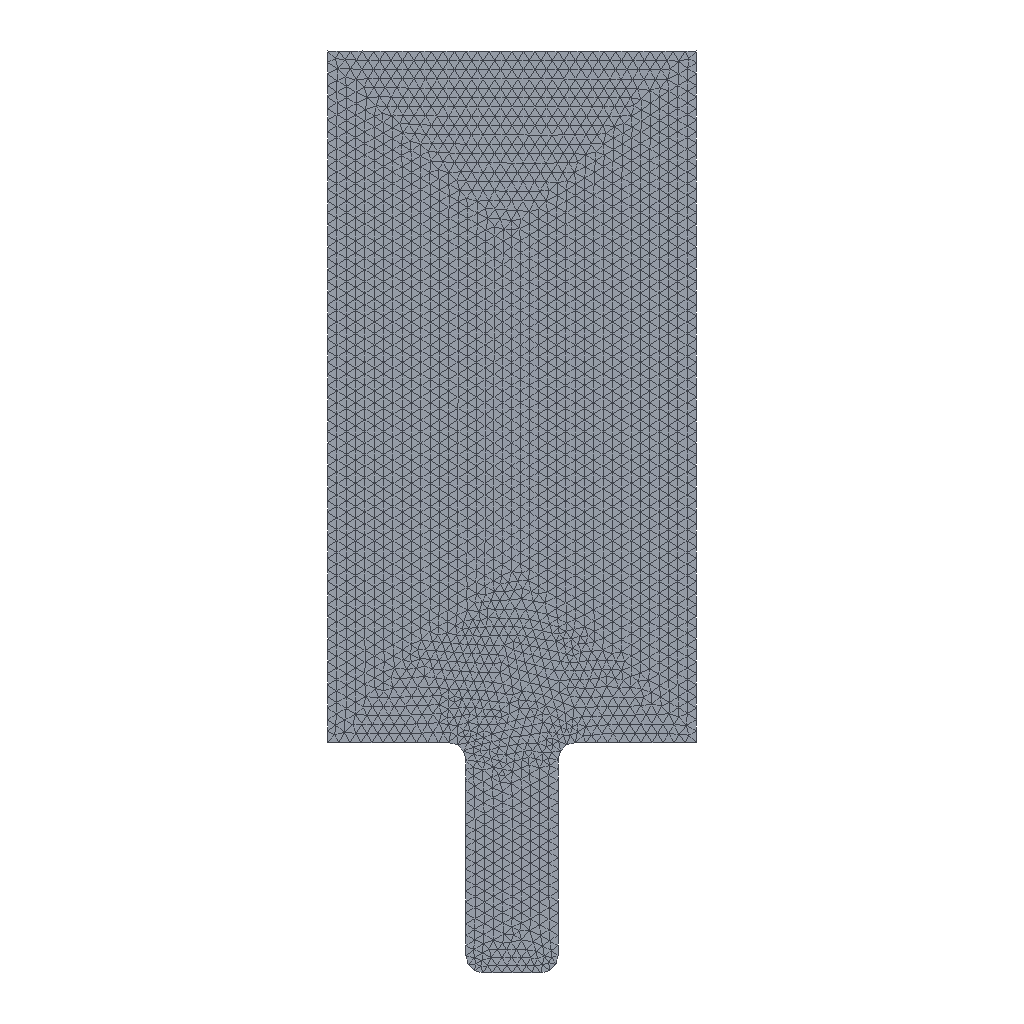Simulation study | comsol
Notes in the study folder:
rho_water 1e3[kg/m^3] Density, water
mu_water 1.002e-3[Pa*s] Dynamic viscosity, water
perm_water 8.0e1[1] Permittivity, water
rho_oil 8.84e2[kg/m^3] Density, oil
mu_oil 4.74e-1[Pa*s] Dynamic viscosity, oil
perm_oil 2.2[1] Permittivity, oil
Notes in the study folder:
epsilon_r tpf.Vf1*perm_water+tpf.Vf2*perm_oil Phase dependent permittivity
Tem11 -epsilon0_const*epsilon_r/2*(es.Ex^2+es.Ey^2)+epsilon0_const*epsilon_r*es.Ex^2 Maxwell stress tensor, 11-component
Tem22 -epsilon0_const*epsilon_r/2*(es.Ex^2+es.Ey^2)+epsilon0_const*epsilon_r*es.Ey^2 Maxwell stress tensor, 22-component
Tem12 epsilon0_const*epsilon_r*es.Ex*es.Ey Maxwell stress tensor, 12-component
Tem21 epsilon0_const*epsilon_r*es.Ex*es.Ey Maxwell stress tensor, 21-component
Fx d(Tem11,x)+d(Tem12,y) Force, x-component
Fy d(Tem21,x)+d(Tem22,y) Force, y-component
Set-up summary:
category,name,step,type,value,unit,region
solver,comsol,,COMSOL Multiphysics 6.4 (Build: 293)
units,SI; geometry length unit m,,stated,COMSOL default unit system (SI)
analysis,Study 1,,Transient,space_dimension=2D
load_step,std1/time,std1/time,Transient,"type=Transient; times=range(0,0.1,5)"
mesh,nodes,,,2852
mesh,elements,,,5474
element_type,tri,,,5474
element_type,edg,,,228
element_type,vtx,,,12
component,mod1,,2D,geometry=geom1; domains=1
physics,Nernst-Planck Equations (chnp),mod1,NernstPlanck,"c1(c1 c2), V(V)"
physics,Moving Mesh (ale),mod1,MovingMesh
parameter,Cinit,,,500[mol/(m^3)]
parameter,T0,,,298[K]
parameter,i0,,,150[A/m^2]
parameter,phi_eq,,,0[V]
parameter,alpha,,,0.75[1]
parameter,phi_s_anode,,,0.0859[V]
parameter,phi_s_cathode,,,-0.0859[V]
parameter,z_net,,,2[1]
parameter,z_c1,,,z_net[1]
parameter,z_c2,,,-z_net[1]
parameter,um_c1,,,D_c1/R_const/T0
parameter,um_c2,,,um_c1
parameter,MCu,,,63.546e-3[kg/mol]
parameter,rhoCu,,,7.7264e3[kg/m^3]
parameter,D_c1,,,2e-9[m^2/s]
parameter,alpha1,,,0.5[1]
parameter,alpha2,,,1.5[1]
parameter,D_c2,,,D_c1
bc,Species Charges (sp1),mod1/chnp,SpeciesProperties,z=z_c1 z_c2; a0=0.4[nm] 0.4[nm]; a0H=0.9[nm]; a0OH=0.3[nm]; f=1 1; fH=1; fOH=1,,selection [1]
bc,"Convection, Diffusion, and Migration 1 (cdm1)",mod1/chnp,Fluid,u=0 0 0; um=um_c1 um_c2; MobilityModel=UserDefined; D_c1=D_c1; D_c2=D_c2; DiffusionCoefficientSource=mat; Dm_c1=1e-9[m^2/s]; DiffusionMaterialList=none; Dchem_c1=1e-9[m^2/s]; DH=9.3e-9[m^2/s]; DOH=5.3e-9[m^2/s]; Dm_c2=1e-9[m^2/s]; Dchem_c2=1e-9[m^2/s]; umH=3.8e-12[s*mol/kg]; umOH=2.2e-12[s*mol/kg]; epsilonr=80,,selection [1]
bc,Electric Insulation 1 (ein1),mod1/chnp,ElectricInsulation,,,"selection [1, 8]"
bc,No Flux 1 (nflx1),mod1/chnp,NoFlux,IncludeConvection=1,,"selection [1, 2, 3, 4, 5, 6, 7, 8, 9, 10, 11, 12]"
bc,Initial Values 1 (init1),mod1/chnp,init,initc=0 Cinit; initV=(-0.01+0.02*Y/(4e-5[m]))*1[V],,selection [1]
bc,Continuity (dcont1),mod1/chnp,Continuity,pairDisconnect=1; pairSelection=all; pairsList=0,,selection []
bc,Current Density 1 (cdens1),mod1/chnp,CurrentDensity,i0=i_cathode,,"selection [2, 4, 5, 6, 7, 9, 10, 11, 12]"
bc,Current Density 2 (cdens2),mod1/chnp,CurrentDensity,i0=i_anode,,selection [3]
bc,Fixed Mesh 1 (fix1),mod1/ale,FixedMesh,,,selection []
bc,Prescribed Mesh Displacement 1 (disp1),mod1/ale,PrescribedMeshDisplacement,useDx=1 1; dx=0 0; weakConstraints=0,,selection []
bc,Free Deformation 1 (free1),mod1/ale,FreeDeformation,dxInit=0 0,,selection [1]
bc,Prescribed Mesh Velocity 1 (vel1),mod1/ale,PrescribedMeshVelocity,useVx=1 1; vx=n_growth*chnp.nx n_growth*chnp.ny; weakConstraints=0,,selection [3]
bc,Prescribed Mesh Velocity 2 (vel2),mod1/ale,PrescribedMeshVelocity,useVx=1 1; vx=growth*chnp.nx growth*chnp.ny; weakConstraints=0,,"selection [2, 4, 5, 6, 7, 9, 10, 11, 12]"
bc,Prescribed Mesh Displacement 2 (disp2),mod1/ale,PrescribedMeshDisplacement,useDx=1 0; dx=0 0; weakConstraints=0,,"selection [1, 8]"
COMSOL model file for Java, long lists of numbers shortened:
/*
 * em_deck.java
 */

import com.comsol.model.*;
import com.comsol.model.util.*;

/** Model exported on Oct 28 2026, 10:35 by COMSOL 6.4.0.293. */
public class em_deck {

  public static Model run() {
    Model model = ModelUtil.create("Model");

    model.modelPath("");

    model.label("in.mph");

    model.param().set("Cinit", "500[mol/(m^3)]", "Initial concentration");
    model.param().set("T0", "298[K]", "System temperature");
    model.param().set("i0", "150[A/m^2]", "Exchange current density");
    model.param().set("phi_eq", "0[V]", "Relative equilibrium potential");
    model.param().set("alpha", "0.75[1]", "Symmetry factor");
    model.param().set("phi_s_anode", "0.0859[V]", "Anode potential");
    model.param().set("phi_s_cathode", "-0.0859[V]", "Cathode potential");
    model.param().set("z_net", "2[1]", "Net species charge");
    model.param().set("z_c1", "z_net[1]", "Charge, species c1");
    model.param().set("z_c2", "-z_net[1]", "Charge, species c2");
    model.param().set("um_c1", "D_c1/R_const/T0", "Mobility, species c1");
    model.param().set("um_c2", "um_c1", "Mobility, species c2");
    model.param().set("MCu", "63.546e-3[kg/mol]", "Cu molar mass");
    model.param().set("rhoCu", "7.7264e3[kg/m^3]", "Cu density");
    model.param().set("D_c1", "2e-9[m^2/s]", "Diffusivity");
    model.param().set("alpha1", "0.5[1]", "Symmetry factor");
    model.param().set("alpha2", "1.5[1]", "Diffusivity");
    model.param().set("D_c2", "D_c1", "Symmetry factor");

    model.component().create("mod1", false);

    model.component("mod1").geom().create("geom1", 2);

    model.component("mod1").label("Model 1");

    model.component("mod1").defineLocalCoord(false);

    model.component("mod1").curvedInterior(false);

    model.component("mod1").mesh().create("mesh1");

    model.component("mod1").geom("geom1").repairTolType("relative");
    model.component("mod1").geom("geom1").create("r1", "Rectangle");
    model.component("mod1").geom("geom1").feature("r1").set("size", new String[]{"1.6e-5", "3e-5"});
    model.component("mod1").geom("geom1").feature("r1").set("pos", new String[]{"-0.8e-5", "1e-5"});
    model.component("mod1").geom("geom1").create("r2", "Rectangle");
    model.component("mod1").geom("geom1").feature("r2").set("size", new String[]{"0.4e-5", "1e-5"});
    model.component("mod1").geom("geom1").feature("r2").set("pos", new String[]{"-0.2e-5", "0"});
    model.component("mod1").geom("geom1").create("uni1", "Union");
    model.component("mod1").geom("geom1").feature("uni1").set("intbnd", false);
    model.component("mod1").geom("geom1").feature("uni1").selection("input").set("r1", "r2");
    model.component("mod1").geom("geom1").create("fil1", "Fillet");
    model.component("mod1").geom("geom1").feature("fil1").set("radius", "7.5e-7");
    model.component("mod1").geom("geom1").feature("fil1").selection("point").set("uni1(1)", 3, 4, 5, 6);
    model.component("mod1").geom("geom1").feature("fin").set("repairtoltype", "relative");
    model.component("mod1").geom("geom1").run();

    model.component("mod1").selection().create("sel1", "Explicit");
    model.component("mod1").selection("sel1").geom("geom1", 1);
    model.component("mod1").selection("sel1").set(3);
    model.component("mod1").selection().create("sel2", "Explicit");
    model.component("mod1").selection("sel2").geom("geom1", 1);
    model.component("mod1").selection("sel2").set(2, 4, 5, 6, 7, 9, 10, 11, 12);
    model.component("mod1").selection("sel1").label("anode");
    model.component("mod1").selection("sel2").label("cathode");

    model.component("mod1").variable().create("var1");
    model.component("mod1").variable("var1")
         .set("i_anode", "i0*(exp(alpha*z_net*F_const/R_const/T0*(phi_s_anode-V-phi_eq))-c1/Cinit*exp(-alpha1*z_net*F_const/R_const/T0*(phi_s_anode-V-phi_eq)))", "Anode current density");
    model.component("mod1").variable("var1")
         .set("i_cathode", "i0*(exp(alpha2*z_net*F_const/R_const/T0*(phi_s_cathode-V-phi_eq))-c1/Cinit*exp(-alpha1*z_net*F_const/R_const/T0*(phi_s_cathode-V-phi_eq)))", "Cathode current density");
    model.component("mod1").variable("var1")
         .set("growth", "i_cathode*MCu/rhoCu/z_net/F_const", "Deposition rate, cathode");
    model.component("mod1").variable("var1")
         .set("n_growth", "i_anode*MCu/rhoCu/z_net/F_const", "Deposition rate, anode");
    model.component("mod1").variable("var1").set("displ_x", "abs(x-X)", "Absolute displacement in x direction");

    model.component("mod1").physics().create("chnp", "NernstPlanck", "geom1");
    model.component("mod1").physics("chnp").identifier("chnp");
    model.component("mod1").physics("chnp").create("cdens1", "CurrentDensity", 1);
    model.component("mod1").physics("chnp").feature("cdens1").selection().named("sel2");
    model.component("mod1").physics("chnp").create("cdens2", "CurrentDensity", 1);
    model.component("mod1").physics("chnp").feature("cdens2").selection().named("sel1");
    model.component("mod1").physics().create("ale", "MovingMesh", "geom1");
    model.component("mod1").physics("ale").create("free1", "FreeDeformation", 2);
    model.component("mod1").physics("ale").feature("free1").selection().set(1);
    model.component("mod1").physics("ale").create("vel1", "PrescribedMeshVelocity", 1);
    model.component("mod1").physics("ale").feature("vel1").selection().named("sel1");
    model.component("mod1").physics("ale").create("vel2", "PrescribedMeshVelocity", 1);
    model.component("mod1").physics("ale").feature("vel2").selection().named("sel2");
    model.component("mod1").physics("ale").create("disp2", "PrescribedMeshDisplacement", 1);
    model.component("mod1").physics("ale").feature("disp2").selection().set(1, 8);

    model.component("mod1").mesh("mesh1").create("ftri1", "FreeTri");

    model.thermodynamics().label("Thermodynamics Package");

    model.component("mod1").view("view1").set("showlabels", true);
    model.component("mod1").view("view1").axis().set("xmin", -1.8310764988070464E-5);
    model.component("mod1").view("view1").axis().set("xmax", 1.8310764988070464E-5);
    model.component("mod1").view("view1").axis().set("ymin", -3.7111165056558093E-6);
    model.component("mod1").view("view1").axis().set("ymax", 4.537731729215011E-5);

    model.component("mod1").physics("chnp").label("Nernst-Planck Equations");
    model.component("mod1").physics("chnp").prop("ShapeProperty").set("boundaryFlux_concentration", false);
    model.component("mod1").physics("chnp").prop("ShapeProperty").set("boundaryFlux_electricpotential", false);
    model.component("mod1").physics("chnp").prop("MassConsistentStabilization").set("CrosswindType", "Codina");
    model.component("mod1").physics("chnp").prop("AdvancedSettings").set("BackCompState", 0);
    model.component("mod1").physics("chnp").feature("sp1").set("z", new String[][]{{"z_c1"}, {"z_c2"}});
    model.component("mod1").physics("chnp").feature("sp1").label("Species Charges");
    model.component("mod1").physics("chnp").feature("cdm1")
         .set("um", new String[][]{{"um_c1", "0", "0", "0", "um_c1", "0", "0", "0", "um_c1"},
         {"um_c2", "0", "0", "0", "um_c2", "0", "0", "0", "um_c2"}});
    model.component("mod1").physics("chnp").feature("cdm1").set("minput_temperature_src", "userdef");
    model.component("mod1").physics("chnp").feature("cdm1").set("minput_strainreferencetemperature", 0);
    model.component("mod1").physics("chnp").feature("cdm1").set("minput_concentration_src", "root.mod1.c2");
    model.component("mod1").physics("chnp").feature("cdm1").set("MobilityModel", "UserDefined");
    model.component("mod1").physics("chnp").feature("cdm1")
         .set("D_c1", new String[][]{{"D_c1"}, {"0"}, {"0"}, {"0"}, {"D_c1"}, {"0"}, {"0"}, {"0"}, {"D_c1"}});
    model.component("mod1").physics("chnp").feature("cdm1")
         .set("D_c2", new String[][]{{"D_c2"}, {"0"}, {"0"}, {"0"}, {"D_c2"}, {"0"}, {"0"}, {"0"}, {"D_c2"}});
    model.component("mod1").physics("chnp").feature("cdm1").label("Convection, Diffusion, and Migration 1");
    model.component("mod1").physics("chnp").feature("nflx1").set("IncludeConvection", true);
    model.component("mod1").physics("chnp").feature("init1").set("initc", new String[][]{{"0"}, {"Cinit"}});
    model.component("mod1").physics("chnp").feature("init1").set("initV", "(-0.01+0.02*Y/(4e-5[m]))*1[V]");
    model.component("mod1").physics("chnp").feature("dcont1").set("pairDisconnect", true);
    model.component("mod1").physics("chnp").feature("dcont1").label("Continuity");
    model.component("mod1").physics("chnp").feature("cdens1").set("i0", "i_cathode");
    model.component("mod1").physics("chnp").feature("cdens2").set("i0", "i_anode");
    model.component("mod1").physics("ale").prop("FrameSettings").set("geometryShapeOrder", 1);
    model.component("mod1").physics("ale").prop("freeDeformationControlsBoundaries")
         .set("freeDeformationControlsBoundaries", 1);
    model.component("mod1").physics("ale").feature("vel1")
         .set("vx", new String[][]{{"n_growth*chnp.nx"}, {"n_growth*chnp.ny"}});
    model.component("mod1").physics("ale").feature("vel2")
         .set("vx", new String[][]{{"growth*chnp.nx"}, {"growth*chnp.ny"}});
    model.component("mod1").physics("ale").feature("disp2").set("useDx", new int[][]{{1}, {0}});

    model.component("mod1").mesh("mesh1").feature("size").set("hauto", 2);
    model.component("mod1").mesh("mesh1").feature("size").set("custom", "on");
    model.component("mod1").mesh("mesh1").feature("size").set("hmax", 5.0E-7);
    model.component("mod1").mesh("mesh1").feature("size").set("hcurve", 0.9);
    model.component("mod1").mesh("mesh1").feature("ftri1").set("smoothcontrol", true);
    model.component("mod1").mesh("mesh1").feature("ftri1").set("smoothmaxiter", 8);
    model.component("mod1").mesh("mesh1").feature("ftri1").set("smoothmaxdepth", 8);
    model.component("mod1").mesh("mesh1").run();

    model.study().create("std1");
    model.study("std1").create("time", "Transient");

    model.sol().create("sol1");
    model.sol("sol1").attach("std1");
    model.sol("sol1").create("st1", "StudyStep");
    model.sol("sol1").create("v1", "Variables");
    model.sol("sol1").create("t1", "Time");
    model.sol("sol1").feature("t1").create("fc1", "FullyCoupled");
    model.sol("sol1").feature("t1").create("d1", "Direct");
    model.sol("sol1").feature("t1").feature().remove("fcDef");

    model.result().dataset().create("dset2", "Solution");
    model.result().create("pg1", "PlotGroup2D");
    model.result().create("pg2", "PlotGroup1D");
    model.result("pg1").create("surf1", "Surface");
    model.result("pg1").create("con1", "Contour");
    model.result("pg1").create("str1", "Streamline");
    model.result("pg1").create("line1", "Line");
    model.result("pg1").feature("con1").set("expr", "V");
    model.result("pg1").feature("str1").set("expr", new String[]{"chnp.tfluxx_c1", "chnp.tfluxy_c1"});
    model.result("pg1").feature("line1").set("data", "dset2");
    model.result("pg2").create("lngr1", "LineGraph");
    model.result("pg2").feature("lngr1").set("xdata", "expr");
    model.result("pg2").feature("lngr1").selection().set(4);
    model.result("pg2").feature("lngr1").set("expr", "mod1.displ_x");

    model.study("std1").feature("time").set("tlist", "range(0,0.1,5)");

    model.sol("sol1").label("Solver 1");
    model.sol("sol1").feature("st1").label("Compile Equations: Time Dependent");
    model.sol("sol1").feature("v1").label("Dependent Variables 1.1");
    model.sol("sol1").feature("v1").set("clistctrl", new String[]{});
    model.sol("sol1").feature("v1").set("cname", new String[]{});
    model.sol("sol1").feature("v1").set("clist", new int[]{});
    model.sol("sol1").feature("t1").label("Time-Dependent Solver 1.1");
    model.sol("sol1").feature("t1").set("tlist", "range(0,0.1,5)");
    model.sol("sol1").feature("t1").set("atolglobalvaluemethod", "manual");
    model.sol("sol1").feature("t1").set("atolglobal", "0.001");
    model.sol("sol1").feature("t1").set("ewtrescale", false);
    model.sol("sol1").feature("t1")
         .set("atolvaluemethod", new String[]{"mod1_V", "manual", "mod1_c2", "manual", "mod1_spatial_disp", "manual"});
    model.sol("sol1").feature("t1").set("initialstepbdf", "0.001");
    model.sol("sol1").feature("t1").set("maxorder", 2);
    model.sol("sol1").feature("t1").set("bwinitstepfrac", "1.0");
    model.sol("sol1").feature("t1").feature("dDef").label("Direct 2");
    model.sol("sol1").feature("t1").feature("dDef").set("thresh", 0.1);
    model.sol("sol1").feature("t1").feature("dDef").set("ooc", false);
    model.sol("sol1").feature("t1").feature("dDef").set("rhob", 400);
    model.sol("sol1").feature("t1").feature("aDef").label("Advanced 1");
    model.sol("sol1").feature("t1").feature("fc1").label("Fully Coupled 1.1");
    model.sol("sol1").feature("t1").feature("fc1").set("maxiter", 5);
    model.sol("sol1").feature("t1").feature("fc1").set("jtech", "once");
    model.sol("sol1").feature("t1").feature("fc1").set("probesel", "manual");
    model.sol("sol1").feature("t1").feature("d1").label("Direct 1.1");
    model.sol("sol1").feature("t1").feature("d1").set("thresh", 0.1);
    model.sol("sol1").feature("t1").feature("d1").set("ooc", false);
    model.sol("sol1").feature("t1").feature("d1").set("rhob", 400);

    model.study("std1").runNoGen();

    model.result().dataset("dset1").label("Solution 1");
    model.result().dataset("dset2").label("Solution 2");
    model.result("pg1").set("smooth", "internal");
    model.result("pg1").feature("surf1").set("descr", "Concentration");
    model.result("pg1").feature("surf1").set("colortable", "RainbowClassic");
    model.result("pg1").feature("surf1").set("smooth", "internal");
    model.result("pg1").feature("surf1").set("resolution", "normal");
    model.result("pg1").feature("con1").set("levelrounding", false);
    model.result("pg1").feature("con1").set("coloring", "uniform");
    model.result("pg1").feature("con1").set("colorlegend", false);
    model.result("pg1").feature("con1").set("color", "black");
    model.result("pg1").feature("con1").set("smooth", "internal");
    model.result("pg1").feature("con1").set("resolution", "normal");
    model.result("pg1").feature("str1").set("descr", "Total flux");
    model.result("pg1").feature("str1").set("posmethod", "magnitude");
    model.result("pg1").feature("str1").set("magdensity", new String[]{"max(0,5+2*log(0.5))", "max(0,5+2*log(29))"});
    model.result("pg1").feature("str1").set("madv", "manual");
    model.result("pg1").feature("str1").set("msatfactor", 1.4);
    model.result("pg1").feature("str1").set("smooth", "internal");
    model.result("pg1").feature("str1").set("resolution", "normal");
    model.result("pg1").feature("line1").set("coloring", "uniform");
    model.result("pg1").feature("line1").set("color", "black");
    model.result("pg1").feature("line1").set("smooth", "internal");
    model.result("pg1").feature("line1").set("resolution", "normal");
    model.result("pg2").set("innerinput", "manual");
    model.result("pg2").set("solnum", new int[]{1, 11, 21, 31, 41, 51});
    model.result("pg2").set("titletype", "manual");
    model.result("pg2").set("title", "Thickness of Deposited Copper");
    model.result("pg2").set("xlabel", "Distance from Cavity Bottom");
    model.result("pg2").set("xlabelactive", true);
    model.result("pg2").set("ylabel", "Thickness of Deposited Copper");
    model.result("pg2").set("ylabelactive", true);
    model.result("pg2").set("smooth", "internal");
    model.result("pg2").feature("lngr1").set("xdataexpr", "Y");
    model.result("pg2").feature("lngr1").set("xdataunit", "m");
    model.result("pg2").feature("lngr1").set("xdatadescr", "Y-Coordinate");
    model.result("pg2").feature("lngr1").set("smooth", "none");
    model.result("pg2").feature("lngr1").set("resolution", "normal");

    return model;
  }

  public static void main(String[] args) {
    run();
  }

}
Results summary:
result,max c1 = sqrt(abs(mod1.c1)^2+abs(mod1.c2)^2),dset1 (51 solution(s)),,973.983,mol/m^3
result,max c1 = sqrt(abs(mod1.c1)^2+abs(mod1.c2)^2),dset2 (51 solution(s)),,973.983,mol/m^3